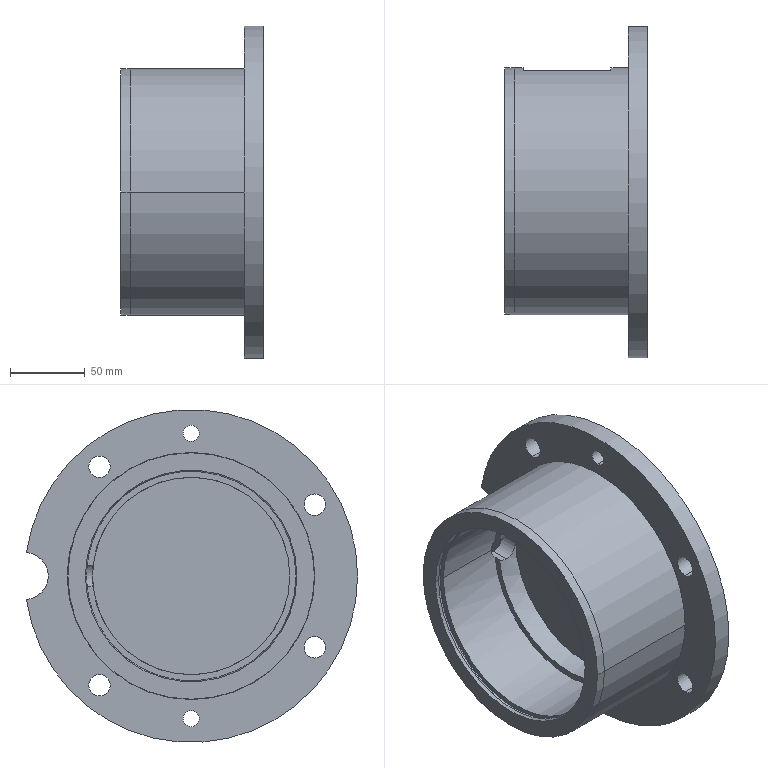Part | SolidWorks | features ICE 3, HoleWzd 2, Fillet 1, Revolution 1 | 1 solid | 44 faces | box 95.25 x 221.134 x 222.25 mm | volume 1161416 mm3 | cylinder 28 | plane 12 | cone 4 | commonest cylinder face diameters 14.287 x8 10.716 x4 140.015 x4 6 x2 19.05 x2 131.826 x2